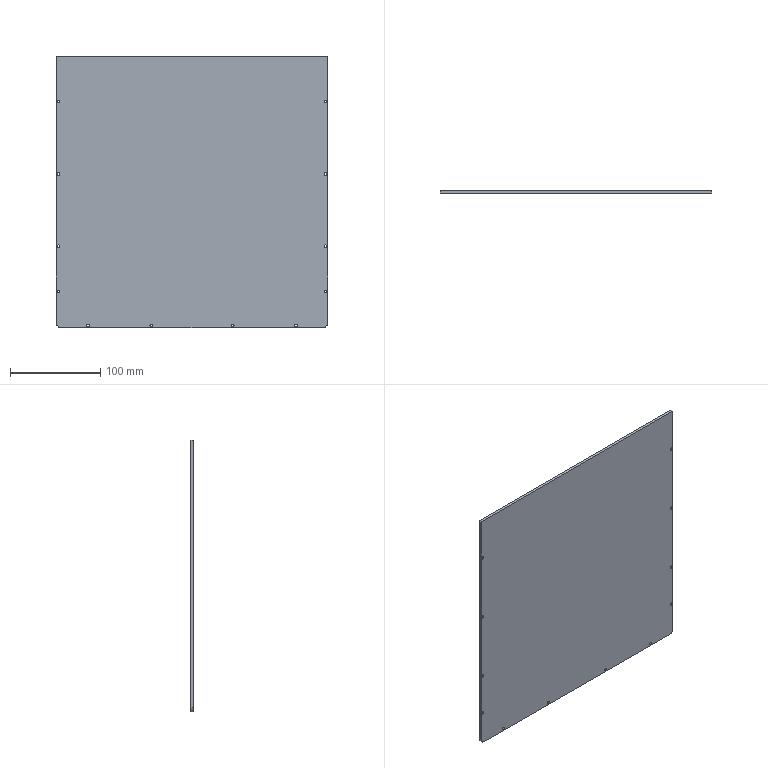Part | SolidWorks | features Extrusion 1 | 1 solid | 32 faces | box 300 x 3 x 300 mm | volume 269713 mm3 | cylinder 26 | plane 6 | commonest cylinder face diameters 3 x24 10 x2
STEP:
#1=CARTESIAN_POINT('',(147.5,3.,-61.5));
#2=VERTEX_POINT('',#1);
#3=CARTESIAN_POINT('',(147.5,3.,-58.5));
#4=VERTEX_POINT('',#3);
#5=CARTESIAN_POINT('',(147.5,3.,-60.));
#6=DIRECTION('',(0.,1.,0.));
#7=DIRECTION('',(0.,0.,-1.));
#8=AXIS2_PLACEMENT_3D('',#5,#6,#7);
#9=CIRCLE('',#8,1.5);
#10=EDGE_CURVE('',#2,#4,#9,.T.);
#11=ORIENTED_EDGE('',*,*,#10,.T.);
#12=CARTESIAN_POINT('',(147.5,0.,-58.5));
#13=VERTEX_POINT('',#12);
#14=CARTESIAN_POINT('',(147.5,3.,-58.5));
#15=DIRECTION('',(0.,-1.,0.));
#16=VECTOR('',#15,1000.);
#17=LINE('',#14,#16);
#18=EDGE_CURVE('',#4,#13,#17,.T.);
#19=ORIENTED_EDGE('',*,*,#18,.T.);
#20=CARTESIAN_POINT('',(147.5,0.,-61.5));
#21=VERTEX_POINT('',#20);
#22=CARTESIAN_POINT('',(147.5,0.,-60.));
#23=DIRECTION('',(0.,1.,0.));
#24=DIRECTION('',(0.,0.,-1.));
#25=AXIS2_PLACEMENT_3D('',#22,#23,#24);
#26=CIRCLE('',#25,1.5);
#27=EDGE_CURVE('',#21,#13,#26,.T.);
#28=ORIENTED_EDGE('',*,*,#27,.F.);
#29=CARTESIAN_POINT('',(147.5,3.,-61.5));
#30=DIRECTION('',(0.,-1.,0.));
#31=VECTOR('',#30,1000.);
#32=LINE('',#29,#31);
#33=EDGE_CURVE('',#2,#21,#32,.T.);
#34=ORIENTED_EDGE('',*,*,#33,.F.);
#35=EDGE_LOOP('',(#11,#19,#28,#34));
#36=FACE_OUTER_BOUND('',#35,.T.);
#37=CARTESIAN_POINT('',(147.5,3.,-60.));
#38=DIRECTION('',(0.,-1.,0.));
#39=DIRECTION('',(0.,0.,-1.));
#40=AXIS2_PLACEMENT_3D('',#37,#38,#39);
#41=CYLINDRICAL_SURFACE('',#40,1.5);
#42=ADVANCED_FACE('',(#36),#41,.F.);
#43=CARTESIAN_POINT('',(147.5,3.,-111.5));
#44=VERTEX_POINT('',#43);
#45=CARTESIAN_POINT('',(147.5,3.,-108.5));
#46=VERTEX_POINT('',#45);
#47=CARTESIAN_POINT('',(147.5,3.,-110.));
#48=DIRECTION('',(0.,1.,0.));
#49=DIRECTION('',(0.,0.,-1.));
#50=AXIS2_PLACEMENT_3D('',#47,#48,#49);
#51=CIRCLE('',#50,1.5);
#52=EDGE_CURVE('',#44,#46,#51,.T.);
#53=ORIENTED_EDGE('',*,*,#52,.T.);
#54=CARTESIAN_POINT('',(147.5,0.,-108.5));
#55=VERTEX_POINT('',#54);
#56=CARTESIAN_POINT('',(147.5,3.,-108.5));
#57=DIRECTION('',(0.,-1.,0.));
#58=VECTOR('',#57,1000.);
#59=LINE('',#56,#58);
#60=EDGE_CURVE('',#46,#55,#59,.T.);
#61=ORIENTED_EDGE('',*,*,#60,.T.);
#62=CARTESIAN_POINT('',(147.5,0.,-111.5));
#63=VERTEX_POINT('',#62);
#64=CARTESIAN_POINT('',(147.5,0.,-110.));
#65=DIRECTION('',(0.,1.,0.));
#66=DIRECTION('',(0.,0.,-1.));
#67=AXIS2_PLACEMENT_3D('',#64,#65,#66);
#68=CIRCLE('',#67,1.5);
#69=EDGE_CURVE('',#63,#55,#68,.T.);
#70=ORIENTED_EDGE('',*,*,#69,.F.);
#71=CARTESIAN_POINT('',(147.5,3.,-111.5));
#72=DIRECTION('',(0.,-1.,0.));
#73=VECTOR('',#72,1000.);
#74=LINE('',#71,#73);
#75=EDGE_CURVE('',#44,#63,#74,.T.);
#76=ORIENTED_EDGE('',*,*,#75,.F.);
#77=EDGE_LOOP('',(#53,#61,#70,#76));
#78=FACE_OUTER_BOUND('',#77,.T.);
#79=CARTESIAN_POINT('',(147.5,3.,-110.));
#80=DIRECTION('',(0.,-1.,0.));
#81=DIRECTION('',(0.,0.,-1.));
#82=AXIS2_PLACEMENT_3D('',#79,#80,#81);
#83=CYLINDRICAL_SURFACE('',#82,1.5);
#84=ADVANCED_FACE('',(#78),#83,.F.);
#85=CARTESIAN_POINT('',(147.5,3.,98.5));
#86=VERTEX_POINT('',#85);
#87=CARTESIAN_POINT('',(147.5,3.,101.5));
#88=VERTEX_POINT('',#87);
#89=CARTESIAN_POINT('',(147.5,3.,100.));
#90=DIRECTION('',(0.,1.,0.));
#91=DIRECTION('',(0.,0.,-1.));
#92=AXIS2_PLACEMENT_3D('',#89,#90,#91);
#93=CIRCLE('',#92,1.5);
#94=EDGE_CURVE('',#86,#88,#93,.T.);
#95=ORIENTED_EDGE('',*,*,#94,.T.);
#96=CARTESIAN_POINT('',(147.5,0.,101.5));
#97=VERTEX_POINT('',#96);
#98=CARTESIAN_POINT('',(147.5,3.,101.5));
#99=DIRECTION('',(0.,-1.,0.));
#100=VECTOR('',#99,1000.);
#101=LINE('',#98,#100);
#102=EDGE_CURVE('',#88,#97,#101,.T.);
#103=ORIENTED_EDGE('',*,*,#102,.T.);
#104=CARTESIAN_POINT('',(147.5,0.,98.5));
#105=VERTEX_POINT('',#104);
#106=CARTESIAN_POINT('',(147.5,0.,100.));
#107=DIRECTION('',(0.,1.,0.));
#108=DIRECTION('',(0.,0.,-1.));
#109=AXIS2_PLACEMENT_3D('',#106,#107,#108);
#110=CIRCLE('',#109,1.5);
#111=EDGE_CURVE('',#105,#97,#110,.T.);
#112=ORIENTED_EDGE('',*,*,#111,.F.);
#113=CARTESIAN_POINT('',(147.5,3.,98.5));
#114=DIRECTION('',(0.,-1.,0.));
#115=VECTOR('',#114,1000.);
#116=LINE('',#113,#115);
#117=EDGE_CURVE('',#86,#105,#116,.T.);
#118=ORIENTED_EDGE('',*,*,#117,.F.);
#119=EDGE_LOOP('',(#95,#103,#112,#118));
#120=FACE_OUTER_BOUND('',#119,.T.);
#121=CARTESIAN_POINT('',(147.5,3.,100.));
#122=DIRECTION('',(0.,-1.,0.));
#123=DIRECTION('',(0.,0.,-1.));
#124=AXIS2_PLACEMENT_3D('',#121,#122,#123);
#125=CYLINDRICAL_SURFACE('',#124,1.5);
#126=ADVANCED_FACE('',(#120),#125,.F.);
#127=CARTESIAN_POINT('',(147.5,3.,18.5));
#128=VERTEX_POINT('',#127);
#129=CARTESIAN_POINT('',(147.5,3.,21.5));
#130=VERTEX_POINT('',#129);
#131=CARTESIAN_POINT('',(147.5,3.,20.));
#132=DIRECTION('',(0.,1.,0.));
#133=DIRECTION('',(0.,0.,-1.));
#134=AXIS2_PLACEMENT_3D('',#131,#132,#133);
#135=CIRCLE('',#134,1.5);
#136=EDGE_CURVE('',#128,#130,#135,.T.);
#137=ORIENTED_EDGE('',*,*,#136,.T.);
#138=CARTESIAN_POINT('',(147.5,0.,21.5));
#139=VERTEX_POINT('',#138);
#140=CARTESIAN_POINT('',(147.5,3.,21.5));
#141=DIRECTION('',(0.,-1.,0.));
#142=VECTOR('',#141,1000.);
#143=LINE('',#140,#142);
#144=EDGE_CURVE('',#130,#139,#143,.T.);
#145=ORIENTED_EDGE('',*,*,#144,.T.);
#146=CARTESIAN_POINT('',(147.5,0.,18.5));
#147=VERTEX_POINT('',#146);
#148=CARTESIAN_POINT('',(147.5,0.,20.));
#149=DIRECTION('',(0.,1.,0.));
#150=DIRECTION('',(0.,0.,-1.));
#151=AXIS2_PLACEMENT_3D('',#148,#149,#150);
#152=CIRCLE('',#151,1.5);
#153=EDGE_CURVE('',#147,#139,#152,.T.);
#154=ORIENTED_EDGE('',*,*,#153,.F.);
#155=CARTESIAN_POINT('',(147.5,3.,18.5));
#156=DIRECTION('',(0.,-1.,0.));
#157=VECTOR('',#156,1000.);
#158=LINE('',#155,#157);
#159=EDGE_CURVE('',#128,#147,#158,.T.);
#160=ORIENTED_EDGE('',*,*,#159,.F.);
#161=EDGE_LOOP('',(#137,#145,#154,#160));
#162=FACE_OUTER_BOUND('',#161,.T.);
#163=CARTESIAN_POINT('',(147.5,3.,20.));
#164=DIRECTION('',(0.,-1.,0.));
#165=DIRECTION('',(0.,0.,-1.));
#166=AXIS2_PLACEMENT_3D('',#163,#164,#165);
#167=CYLINDRICAL_SURFACE('',#166,1.5);
#168=ADVANCED_FACE('',(#162),#167,.F.);
#169=CARTESIAN_POINT('',(115.,3.,-149.));
#170=VERTEX_POINT('',#169);
#171=CARTESIAN_POINT('',(115.,3.,-146.));
#172=VERTEX_POINT('',#171);
#173=CARTESIAN_POINT('',(115.,3.,-147.5));
#174=DIRECTION('',(0.,1.,0.));
#175=DIRECTION('',(0.,0.,-1.));
#176=AXIS2_PLACEMENT_3D('',#173,#174,#175);
#177=CIRCLE('',#176,1.5);
#178=EDGE_CURVE('',#170,#172,#177,.T.);
#179=ORIENTED_EDGE('',*,*,#178,.T.);
#180=CARTESIAN_POINT('',(115.,0.,-146.));
#181=VERTEX_POINT('',#180);
#182=CARTESIAN_POINT('',(115.,3.,-146.));
#183=DIRECTION('',(0.,-1.,0.));
#184=VECTOR('',#183,1000.);
#185=LINE('',#182,#184);
#186=EDGE_CURVE('',#172,#181,#185,.T.);
#187=ORIENTED_EDGE('',*,*,#186,.T.);
#188=CARTESIAN_POINT('',(115.,0.,-149.));
#189=VERTEX_POINT('',#188);
#190=CARTESIAN_POINT('',(115.,0.,-147.5));
#191=DIRECTION('',(0.,1.,0.));
#192=DIRECTION('',(0.,0.,-1.));
#193=AXIS2_PLACEMENT_3D('',#190,#191,#192);
#194=CIRCLE('',#193,1.5);
#195=EDGE_CURVE('',#189,#181,#194,.T.);
#196=ORIENTED_EDGE('',*,*,#195,.F.);
#197=CARTESIAN_POINT('',(115.,3.,-149.));
#198=DIRECTION('',(0.,-1.,0.));
#199=VECTOR('',#198,1000.);
#200=LINE('',#197,#199);
#201=EDGE_CURVE('',#170,#189,#200,.T.);
#202=ORIENTED_EDGE('',*,*,#201,.F.);
#203=EDGE_LOOP('',(#179,#187,#196,#202));
#204=FACE_OUTER_BOUND('',#203,.T.);
#205=CARTESIAN_POINT('',(115.,3.,-147.5));
#206=DIRECTION('',(0.,-1.,0.));
#207=DIRECTION('',(0.,0.,-1.));
#208=AXIS2_PLACEMENT_3D('',#205,#206,#207);
#209=CYLINDRICAL_SURFACE('',#208,1.5);
#210=ADVANCED_FACE('',(#204),#209,.F.);
#211=CARTESIAN_POINT('',(45.,3.,-149.));
#212=VERTEX_POINT('',#211);
#213=CARTESIAN_POINT('',(45.,3.,-146.));
#214=VERTEX_POINT('',#213);
#215=CARTESIAN_POINT('',(45.,3.,-147.5));
#216=DIRECTION('',(0.,1.,0.));
#217=DIRECTION('',(0.,0.,-1.));
#218=AXIS2_PLACEMENT_3D('',#215,#216,#217);
#219=CIRCLE('',#218,1.5);
#220=EDGE_CURVE('',#212,#214,#219,.T.);
#221=ORIENTED_EDGE('',*,*,#220,.T.);
#222=CARTESIAN_POINT('',(45.,0.,-146.));
#223=VERTEX_POINT('',#222);
#224=CARTESIAN_POINT('',(45.,3.,-146.));
#225=DIRECTION('',(0.,-1.,0.));
#226=VECTOR('',#225,1000.);
#227=LINE('',#224,#226);
#228=EDGE_CURVE('',#214,#223,#227,.T.);
#229=ORIENTED_EDGE('',*,*,#228,.T.);
#230=CARTESIAN_POINT('',(45.,0.,-149.));
#231=VERTEX_POINT('',#230);
#232=CARTESIAN_POINT('',(45.,0.,-147.5));
#233=DIRECTION('',(0.,1.,0.));
#234=DIRECTION('',(0.,0.,-1.));
#235=AXIS2_PLACEMENT_3D('',#232,#233,#234);
#236=CIRCLE('',#235,1.5);
#237=EDGE_CURVE('',#231,#223,#236,.T.);
#238=ORIENTED_EDGE('',*,*,#237,.F.);
#239=CARTESIAN_POINT('',(45.,3.,-149.));
#240=DIRECTION('',(0.,-1.,0.));
#241=VECTOR('',#240,1000.);
#242=LINE('',#239,#241);
#243=EDGE_CURVE('',#212,#231,#242,.T.);
#244=ORIENTED_EDGE('',*,*,#243,.F.);
#245=EDGE_LOOP('',(#221,#229,#238,#244));
#246=FACE_OUTER_BOUND('',#245,.T.);
#247=CARTESIAN_POINT('',(45.,3.,-147.5));
#248=DIRECTION('',(0.,-1.,0.));
#249=DIRECTION('',(0.,0.,-1.));
#250=AXIS2_PLACEMENT_3D('',#247,#248,#249);
#251=CYLINDRICAL_SURFACE('',#250,1.5);
#252=ADVANCED_FACE('',(#246),#251,.F.);
#253=CARTESIAN_POINT('',(-45.,3.,-149.));
#254=VERTEX_POINT('',#253);
#255=CARTESIAN_POINT('',(-45.,3.,-146.));
#256=VERTEX_POINT('',#255);
#257=CARTESIAN_POINT('',(-45.,3.,-147.5));
#258=DIRECTION('',(0.,1.,0.));
#259=DIRECTION('',(0.,0.,1.));
#260=AXIS2_PLACEMENT_3D('',#257,#258,#259);
#261=CIRCLE('',#260,1.5);
#262=EDGE_CURVE('',#254,#256,#261,.T.);
#263=ORIENTED_EDGE('',*,*,#262,.T.);
#264=CARTESIAN_POINT('',(-45.,0.,-146.));
#265=VERTEX_POINT('',#264);
#266=CARTESIAN_POINT('',(-45.,3.,-146.));
#267=DIRECTION('',(0.,-1.,0.));
#268=VECTOR('',#267,1000.);
#269=LINE('',#266,#268);
#270=EDGE_CURVE('',#256,#265,#269,.T.);
#271=ORIENTED_EDGE('',*,*,#270,.T.);
#272=CARTESIAN_POINT('',(-45.,0.,-149.));
#273=VERTEX_POINT('',#272);
#274=CARTESIAN_POINT('',(-45.,0.,-147.5));
#275=DIRECTION('',(0.,1.,0.));
#276=DIRECTION('',(0.,0.,1.));
#277=AXIS2_PLACEMENT_3D('',#274,#275,#276);
#278=CIRCLE('',#277,1.5);
#279=EDGE_CURVE('',#273,#265,#278,.T.);
#280=ORIENTED_EDGE('',*,*,#279,.F.);
#281=CARTESIAN_POINT('',(-45.,3.,-149.));
#282=DIRECTION('',(0.,-1.,0.));
#283=VECTOR('',#282,1000.);
#284=LINE('',#281,#283);
#285=EDGE_CURVE('',#254,#273,#284,.T.);
#286=ORIENTED_EDGE('',*,*,#285,.F.);
#287=EDGE_LOOP('',(#263,#271,#280,#286));
#288=FACE_OUTER_BOUND('',#287,.T.);
#289=CARTESIAN_POINT('',(-45.,3.,-147.5));
#290=DIRECTION('',(0.,-1.,0.));
#291=DIRECTION('',(0.,0.,-1.));
#292=AXIS2_PLACEMENT_3D('',#289,#290,#291);
#293=CYLINDRICAL_SURFACE('',#292,1.5);
#294=ADVANCED_FACE('',(#288),#293,.F.);
#295=CARTESIAN_POINT('',(-115.,3.,-149.));
#296=VERTEX_POINT('',#295);
#297=CARTESIAN_POINT('',(-115.,3.,-146.));
#298=VERTEX_POINT('',#297);
#299=CARTESIAN_POINT('',(-115.,3.,-147.5));
#300=DIRECTION('',(0.,1.,0.));
#301=DIRECTION('',(0.,0.,1.));
#302=AXIS2_PLACEMENT_3D('',#299,#300,#301);
#303=CIRCLE('',#302,1.5);
#304=EDGE_CURVE('',#296,#298,#303,.T.);
#305=ORIENTED_EDGE('',*,*,#304,.T.);
#306=CARTESIAN_POINT('',(-115.,0.,-146.));
#307=VERTEX_POINT('',#306);
#308=CARTESIAN_POINT('',(-115.,3.,-146.));
#309=DIRECTION('',(0.,-1.,0.));
#310=VECTOR('',#309,1000.);
#311=LINE('',#308,#310);
#312=EDGE_CURVE('',#298,#307,#311,.T.);
#313=ORIENTED_EDGE('',*,*,#312,.T.);
#314=CARTESIAN_POINT('',(-115.,0.,-149.));
#315=VERTEX_POINT('',#314);
#316=CARTESIAN_POINT('',(-115.,0.,-147.5));
#317=DIRECTION('',(0.,1.,0.));
#318=DIRECTION('',(0.,0.,1.));
#319=AXIS2_PLACEMENT_3D('',#316,#317,#318);
#320=CIRCLE('',#319,1.5);
#321=EDGE_CURVE('',#315,#307,#320,.T.);
#322=ORIENTED_EDGE('',*,*,#321,.F.);
#323=CARTESIAN_POINT('',(-115.,3.,-149.));
#324=DIRECTION('',(0.,-1.,0.));
#325=VECTOR('',#324,1000.);
#326=LINE('',#323,#325);
#327=EDGE_CURVE('',#296,#315,#326,.T.);
#328=ORIENTED_EDGE('',*,*,#327,.F.);
#329=EDGE_LOOP('',(#305,#313,#322,#328));
#330=FACE_OUTER_BOUND('',#329,.T.);
#331=CARTESIAN_POINT('',(-115.,3.,-147.5));
#332=DIRECTION('',(0.,-1.,0.));
#333=DIRECTION('',(0.,0.,-1.));
#334=AXIS2_PLACEMENT_3D('',#331,#332,#333);
#335=CYLINDRICAL_SURFACE('',#334,1.5);
#336=ADVANCED_FACE('',(#330),#335,.F.);
#337=CARTESIAN_POINT('',(-147.5,3.,-111.5));
#338=VERTEX_POINT('',#337);
#339=CARTESIAN_POINT('',(-147.5,3.,-108.5));
#340=VERTEX_POINT('',#339);
#341=CARTESIAN_POINT('',(-147.5,3.,-110.));
#342=DIRECTION('',(0.,1.,0.));
#343=DIRECTION('',(0.,0.,1.));
#344=AXIS2_PLACEMENT_3D('',#341,#342,#343);
#345=CIRCLE('',#344,1.5);
#346=EDGE_CURVE('',#338,#340,#345,.T.);
#347=ORIENTED_EDGE('',*,*,#346,.T.);
#348=CARTESIAN_POINT('',(-147.5,0.,-108.5));
#349=VERTEX_POINT('',#348);
#350=CARTESIAN_POINT('',(-147.5,3.,-108.5));
#351=DIRECTION('',(0.,-1.,0.));
#352=VECTOR('',#351,1000.);
#353=LINE('',#350,#352);
#354=EDGE_CURVE('',#340,#349,#353,.T.);
#355=ORIENTED_EDGE('',*,*,#354,.T.);
#356=CARTESIAN_POINT('',(-147.5,0.,-111.5));
#357=VERTEX_POINT('',#356);
#358=CARTESIAN_POINT('',(-147.5,0.,-110.));
#359=DIRECTION('',(0.,1.,0.));
#360=DIRECTION('',(0.,0.,1.));
#361=AXIS2_PLACEMENT_3D('',#358,#359,#360);
#362=CIRCLE('',#361,1.5);
#363=EDGE_CURVE('',#357,#349,#362,.T.);
#364=ORIENTED_EDGE('',*,*,#363,.F.);
#365=CARTESIAN_POINT('',(-147.5,3.,-111.5));
#366=DIRECTION('',(0.,-1.,0.));
#367=VECTOR('',#366,1000.);
#368=LINE('',#365,#367);
#369=EDGE_CURVE('',#338,#357,#368,.T.);
#370=ORIENTED_EDGE('',*,*,#369,.F.);
#371=EDGE_LOOP('',(#347,#355,#364,#370));
#372=FACE_OUTER_BOUND('',#371,.T.);
#373=CARTESIAN_POINT('',(-147.5,3.,-110.));
#374=DIRECTION('',(0.,-1.,0.));
#375=DIRECTION('',(0.,0.,-1.));
#376=AXIS2_PLACEMENT_3D('',#373,#374,#375);
#377=CYLINDRICAL_SURFACE('',#376,1.5);
#378=ADVANCED_FACE('',(#372),#377,.F.);
#379=CARTESIAN_POINT('',(-147.5,3.,-61.5));
#380=VERTEX_POINT('',#379);
#381=CARTESIAN_POINT('',(-147.5,3.,-58.5));
#382=VERTEX_POINT('',#381);
#383=CARTESIAN_POINT('',(-147.5,3.,-60.));
#384=DIRECTION('',(0.,1.,0.));
#385=DIRECTION('',(0.,0.,1.));
#386=AXIS2_PLACEMENT_3D('',#383,#384,#385);
#387=CIRCLE('',#386,1.5);
#388=EDGE_CURVE('',#380,#382,#387,.T.);
#389=ORIENTED_EDGE('',*,*,#388,.T.);
#390=CARTESIAN_POINT('',(-147.5,0.,-58.5));
#391=VERTEX_POINT('',#390);
#392=CARTESIAN_POINT('',(-147.5,3.,-58.5));
#393=DIRECTION('',(0.,-1.,0.));
#394=VECTOR('',#393,1000.);
#395=LINE('',#392,#394);
#396=EDGE_CURVE('',#382,#391,#395,.T.);
#397=ORIENTED_EDGE('',*,*,#396,.T.);
#398=CARTESIAN_POINT('',(-147.5,0.,-61.5));
#399=VERTEX_POINT('',#398);
#400=CARTESIAN_POINT('',(-147.5,0.,-60.));
#401=DIRECTION('',(0.,1.,0.));
#402=DIRECTION('',(0.,0.,1.));
#403=AXIS2_PLACEMENT_3D('',#400,#401,#402);
#404=CIRCLE('',#403,1.5);
#405=EDGE_CURVE('',#399,#391,#404,.T.);
#406=ORIENTED_EDGE('',*,*,#405,.F.);
#407=CARTESIAN_POINT('',(-147.5,3.,-61.5));
#408=DIRECTION('',(0.,-1.,0.));
#409=VECTOR('',#408,1000.);
#410=LINE('',#407,#409);
#411=EDGE_CURVE('',#380,#399,#410,.T.);
#412=ORIENTED_EDGE('',*,*,#411,.F.);
#413=EDGE_LOOP('',(#389,#397,#406,#412));
#414=FACE_OUTER_BOUND('',#413,.T.);
#415=CARTESIAN_POINT('',(-147.5,3.,-60.));
#416=DIRECTION('',(0.,-1.,0.));
#417=DIRECTION('',(0.,0.,-1.));
#418=AXIS2_PLACEMENT_3D('',#415,#416,#417);
#419=CYLINDRICAL_SURFACE('',#418,1.5);
#420=ADVANCED_FACE('',(#414),#419,.F.);
#421=CARTESIAN_POINT('',(-147.5,3.,18.5));
#422=VERTEX_POINT('',#421);
#423=CARTESIAN_POINT('',(-147.5,3.,21.5));
#424=VERTEX_POINT('',#423);
#425=CARTESIAN_POINT('',(-147.5,3.,20.));
#426=DIRECTION('',(0.,1.,0.));
#427=DIRECTION('',(0.,0.,1.));
#428=AXIS2_PLACEMENT_3D('',#425,#426,#427);
#429=CIRCLE('',#428,1.5);
#430=EDGE_CURVE('',#422,#424,#429,.T.);
#431=ORIENTED_EDGE('',*,*,#430,.T.);
#432=CARTESIAN_POINT('',(-147.5,0.,21.5));
#433=VERTEX_POINT('',#432);
#434=CARTESIAN_POINT('',(-147.5,3.,21.5));
#435=DIRECTION('',(0.,-1.,0.));
#436=VECTOR('',#435,1000.);
#437=LINE('',#434,#436);
#438=EDGE_CURVE('',#424,#433,#437,.T.);
#439=ORIENTED_EDGE('',*,*,#438,.T.);
#440=CARTESIAN_POINT('',(-147.5,0.,18.5));
#441=VERTEX_POINT('',#440);
#442=CARTESIAN_POINT('',(-147.5,0.,20.));
#443=DIRECTION('',(0.,1.,0.));
#444=DIRECTION('',(0.,0.,1.));
#445=AXIS2_PLACEMENT_3D('',#442,#443,#444);
#446=CIRCLE('',#445,1.5);
#447=EDGE_CURVE('',#441,#433,#446,.T.);
#448=ORIENTED_EDGE('',*,*,#447,.F.);
#449=CARTESIAN_POINT('',(-147.5,3.,18.5));
#450=DIRECTION('',(0.,-1.,0.));
#451=VECTOR('',#450,1000.);
#452=LINE('',#449,#451);
#453=EDGE_CURVE('',#422,#441,#452,.T.);
#454=ORIENTED_EDGE('',*,*,#453,.F.);
#455=EDGE_LOOP('',(#431,#439,#448,#454));
#456=FACE_OUTER_BOUND('',#455,.T.);
#457=CARTESIAN_POINT('',(-147.5,3.,20.));
#458=DIRECTION('',(0.,-1.,0.));
#459=DIRECTION('',(0.,0.,-1.));
#460=AXIS2_PLACEMENT_3D('',#457,#458,#459);
#461=CYLINDRICAL_SURFACE('',#460,1.5);
#462=ADVANCED_FACE('',(#456),#461,.F.);
#463=CARTESIAN_POINT('',(-147.5,3.,98.5));
#464=VERTEX_POINT('',#463);
#465=CARTESIAN_POINT('',(-147.5,3.,101.5));
#466=VERTEX_POINT('',#465);
#467=CARTESIAN_POINT('',(-147.5,3.,100.));
#468=DIRECTION('',(0.,1.,0.));
#469=DIRECTION('',(0.,0.,1.));
#470=AXIS2_PLACEMENT_3D('',#467,#468,#469);
#471=CIRCLE('',#470,1.5);
#472=EDGE_CURVE('',#464,#466,#471,.T.);
#473=ORIENTED_EDGE('',*,*,#472,.T.);
#474=CARTESIAN_POINT('',(-147.5,0.,101.5));
#475=VERTEX_POINT('',#474);
#476=CARTESIAN_POINT('',(-147.5,3.,101.5));
#477=DIRECTION('',(0.,-1.,0.));
#478=VECTOR('',#477,1000.);
#479=LINE('',#476,#478);
#480=EDGE_CURVE('',#466,#475,#479,.T.);
#481=ORIENTED_EDGE('',*,*,#480,.T.);
#482=CARTESIAN_POINT('',(-147.5,0.,98.5));
#483=VERTEX_POINT('',#482);
#484=CARTESIAN_POINT('',(-147.5,0.,100.));
#485=DIRECTION('',(0.,1.,0.));
#486=DIRECTION('',(0.,0.,1.));
#487=AXIS2_PLACEMENT_3D('',#484,#485,#486);
#488=CIRCLE('',#487,1.5);
#489=EDGE_CURVE('',#483,#475,#488,.T.);
#490=ORIENTED_EDGE('',*,*,#489,.F.);
#491=CARTESIAN_POINT('',(-147.5,3.,98.5));
#492=DIRECTION('',(0.,-1.,0.));
#493=VECTOR('',#492,1000.);
#494=LINE('',#491,#493);
#495=EDGE_CURVE('',#464,#483,#494,.T.);
#496=ORIENTED_EDGE('',*,*,#495,.F.);
#497=EDGE_LOOP('',(#473,#481,#490,#496));
#498=FACE_OUTER_BOUND('',#497,.T.);
#499=CARTESIAN_POINT('',(-147.5,3.,100.));
#500=DIRECTION('',(0.,-1.,0.));
#501=DIRECTION('',(0.,0.,-1.));
#502=AXIS2_PLACEMENT_3D('',#499,#500,#501);
#503=CYLINDRICAL_SURFACE('',#502,1.5);
#504=ADVANCED_FACE('',(#498),#503,.F.);
#505=CARTESIAN_POINT('',(-150.,3.,-145.));
#506=VERTEX_POINT('',#505);
#507=CARTESIAN_POINT('',(-150.,3.,150.));
#508=VERTEX_POINT('',#507);
#509=CARTESIAN_POINT('',(-150.,3.,150.));
#510=DIRECTION('',(0.,0.,1.));
#511=VECTOR('',#510,1000.);
#512=LINE('',#509,#511);
#513=EDGE_CURVE('',#506,#508,#512,.T.);
#514=ORIENTED_EDGE('',*,*,#513,.T.);
#515=CARTESIAN_POINT('',(150.,3.,150.));
#516=VERTEX_POINT('',#515);
#517=CARTESIAN_POINT('',(-150.,3.,150.));
#518=DIRECTION('',(1.,0.,0.));
#519=VECTOR('',#518,1000.);
#520=LINE('',#517,#519);
#521=EDGE_CURVE('',#508,#516,#520,.T.);
#522=ORIENTED_EDGE('',*,*,#521,.T.);
#523=CARTESIAN_POINT('',(150.,3.,-145.));
#524=VERTEX_POINT('',#523);
#525=CARTESIAN_POINT('',(150.,3.,150.));
#526=DIRECTION('',(0.,0.,-1.));
#527=VECTOR('',#526,1000.);
#528=LINE('',#525,#527);
#529=EDGE_CURVE('',#516,#524,#528,.T.);
#530=ORIENTED_EDGE('',*,*,#529,.T.);
#531=CARTESIAN_POINT('',(145.,3.,-150.));
#532=VERTEX_POINT('',#531);
#533=CARTESIAN_POINT('',(145.,3.,-145.));
#534=DIRECTION('',(0.,1.,0.));
#535=DIRECTION('',(0.,0.,-1.));
#536=AXIS2_PLACEMENT_3D('',#533,#534,#535);
#537=CIRCLE('',#536,5.);
#538=EDGE_CURVE('',#524,#532,#537,.T.);
#539=ORIENTED_EDGE('',*,*,#538,.T.);
#540=CARTESIAN_POINT('',(-145.,3.,-150.));
#541=VERTEX_POINT('',#540);
#542=CARTESIAN_POINT('',(-145.,3.,-150.));
#543=DIRECTION('',(-1.,0.,0.));
#544=VECTOR('',#543,1000.);
#545=LINE('',#542,#544);
#546=EDGE_CURVE('',#532,#541,#545,.T.);
#547=ORIENTED_EDGE('',*,*,#546,.T.);
#548=CARTESIAN_POINT('',(-145.,3.,-145.));
#549=DIRECTION('',(0.,1.,0.));
#550=DIRECTION('',(0.,0.,-1.));
#551=AXIS2_PLACEMENT_3D('',#548,#549,#550);
#552=CIRCLE('',#551,5.);
#553=EDGE_CURVE('',#541,#506,#552,.T.);
#554=ORIENTED_EDGE('',*,*,#553,.T.);
#555=EDGE_LOOP('',(#514,#522,#530,#539,#547,#554));
#556=FACE_OUTER_BOUND('',#555,.T.);
#557=ORIENTED_EDGE('',*,*,#472,.F.);
#558=CARTESIAN_POINT('',(-147.5,3.,100.));
#559=DIRECTION('',(0.,1.,0.));
#560=DIRECTION('',(0.,0.,1.));
#561=AXIS2_PLACEMENT_3D('',#558,#559,#560);
#562=CIRCLE('',#561,1.5);
#563=EDGE_CURVE('',#466,#464,#562,.T.);
#564=ORIENTED_EDGE('',*,*,#563,.F.);
#565=EDGE_LOOP('',(#557,#564));
#566=FACE_BOUND('',#565,.T.);
#567=ORIENTED_EDGE('',*,*,#430,.F.);
#568=CARTESIAN_POINT('',(-147.5,3.,20.));
#569=DIRECTION('',(0.,1.,0.));
#570=DIRECTION('',(0.,0.,1.));
#571=AXIS2_PLACEMENT_3D('',#568,#569,#570);
#572=CIRCLE('',#571,1.5);
#573=EDGE_CURVE('',#424,#422,#572,.T.);
#574=ORIENTED_EDGE('',*,*,#573,.F.);
#575=EDGE_LOOP('',(#567,#574));
#576=FACE_BOUND('',#575,.T.);
#577=ORIENTED_EDGE('',*,*,#388,.F.);
#578=CARTESIAN_POINT('',(-147.5,3.,-60.));
#579=DIRECTION('',(0.,1.,0.));
#580=DIRECTION('',(0.,0.,1.));
#581=AXIS2_PLACEMENT_3D('',#578,#579,#580);
#582=CIRCLE('',#581,1.5);
#583=EDGE_CURVE('',#382,#380,#582,.T.);
#584=ORIENTED_EDGE('',*,*,#583,.F.);
#585=EDGE_LOOP('',(#577,#584));
#586=FACE_BOUND('',#585,.T.);
#587=ORIENTED_EDGE('',*,*,#346,.F.);
#588=CARTESIAN_POINT('',(-147.5,3.,-110.));
#589=DIRECTION('',(0.,1.,0.));
#590=DIRECTION('',(0.,0.,1.));
#591=AXIS2_PLACEMENT_3D('',#588,#589,#590);
#592=CIRCLE('',#591,1.5);
#593=EDGE_CURVE('',#340,#338,#592,.T.);
#594=ORIENTED_EDGE('',*,*,#593,.F.);
#595=EDGE_LOOP('',(#587,#594));
#596=FACE_BOUND('',#595,.T.);
#597=ORIENTED_EDGE('',*,*,#304,.F.);
#598=CARTESIAN_POINT('',(-115.,3.,-147.5));
#599=DIRECTION('',(0.,1.,0.));
#600=DIRECTION('',(0.,0.,1.));
#601=AXIS2_PLACEMENT_3D('',#598,#599,#600);
#602=CIRCLE('',#601,1.5);
#603=EDGE_CURVE('',#298,#296,#602,.T.);
#604=ORIENTED_EDGE('',*,*,#603,.F.);
#605=EDGE_LOOP('',(#597,#604));
#606=FACE_BOUND('',#605,.T.);
#607=ORIENTED_EDGE('',*,*,#262,.F.);
#608=CARTESIAN_POINT('',(-45.,3.,-147.5));
#609=DIRECTION('',(0.,1.,0.));
#610=DIRECTION('',(0.,0.,1.));
#611=AXIS2_PLACEMENT_3D('',#608,#609,#610);
#612=CIRCLE('',#611,1.5);
#613=EDGE_CURVE('',#256,#254,#612,.T.);
#614=ORIENTED_EDGE('',*,*,#613,.F.);
#615=EDGE_LOOP('',(#607,#614));
#616=FACE_BOUND('',#615,.T.);
#617=ORIENTED_EDGE('',*,*,#220,.F.);
#618=CARTESIAN_POINT('',(45.,3.,-147.5));
#619=DIRECTION('',(0.,1.,0.));
#620=DIRECTION('',(0.,0.,-1.));
#621=AXIS2_PLACEMENT_3D('',#618,#619,#620);
#622=CIRCLE('',#621,1.5);
#623=EDGE_CURVE('',#214,#212,#622,.T.);
#624=ORIENTED_EDGE('',*,*,#623,.F.);
#625=EDGE_LOOP('',(#617,#624));
#626=FACE_BOUND('',#625,.T.);
#627=ORIENTED_EDGE('',*,*,#178,.F.);
#628=CARTESIAN_POINT('',(115.,3.,-147.5));
#629=DIRECTION('',(0.,1.,0.));
#630=DIRECTION('',(0.,0.,-1.));
#631=AXIS2_PLACEMENT_3D('',#628,#629,#630);
#632=CIRCLE('',#631,1.5);
#633=EDGE_CURVE('',#172,#170,#632,.T.);
#634=ORIENTED_EDGE('',*,*,#633,.F.);
#635=EDGE_LOOP('',(#627,#634));
#636=FACE_BOUND('',#635,.T.);
#637=ORIENTED_EDGE('',*,*,#136,.F.);
#638=CARTESIAN_POINT('',(147.5,3.,20.));
#639=DIRECTION('',(0.,1.,0.));
#640=DIRECTION('',(0.,0.,-1.));
#641=AXIS2_PLACEMENT_3D('',#638,#639,#640);
#642=CIRCLE('',#641,1.5);
#643=EDGE_CURVE('',#130,#128,#642,.T.);
#644=ORIENTED_EDGE('',*,*,#643,.F.);
#645=EDGE_LOOP('',(#637,#644));
#646=FACE_BOUND('',#645,.T.);
#647=ORIENTED_EDGE('',*,*,#94,.F.);
#648=CARTESIAN_POINT('',(147.5,3.,100.));
#649=DIRECTION('',(0.,1.,0.));
#650=DIRECTION('',(0.,0.,-1.));
#651=AXIS2_PLACEMENT_3D('',#648,#649,#650);
#652=CIRCLE('',#651,1.5);
#653=EDGE_CURVE('',#88,#86,#652,.T.);
#654=ORIENTED_EDGE('',*,*,#653,.F.);
#655=EDGE_LOOP('',(#647,#654));
#656=FACE_BOUND('',#655,.T.);
#657=ORIENTED_EDGE('',*,*,#52,.F.);
#658=CARTESIAN_POINT('',(147.5,3.,-110.));
#659=DIRECTION('',(0.,1.,0.));
#660=DIRECTION('',(0.,0.,-1.));
#661=AXIS2_PLACEMENT_3D('',#658,#659,#660);
#662=CIRCLE('',#661,1.5);
#663=EDGE_CURVE('',#46,#44,#662,.T.);
#664=ORIENTED_EDGE('',*,*,#663,.F.);
#665=EDGE_LOOP('',(#657,#664));
#666=FACE_BOUND('',#665,.T.);
#667=ORIENTED_EDGE('',*,*,#10,.F.);
#668=CARTESIAN_POINT('',(147.5,3.,-60.));
#669=DIRECTION('',(0.,1.,0.));
#670=DIRECTION('',(0.,0.,-1.));
#671=AXIS2_PLACEMENT_3D('',#668,#669,#670);
#672=CIRCLE('',#671,1.5);
#673=EDGE_CURVE('',#4,#2,#672,.T.);
#674=ORIENTED_EDGE('',*,*,#673,.F.);
#675=EDGE_LOOP('',(#667,#674));
#676=FACE_BOUND('',#675,.T.);
#677=CARTESIAN_POINT('',(-145.,3.,-145.));
#678=DIRECTION('',(0.,-1.,0.));
#679=DIRECTION('',(0.,0.,-1.));
#680=AXIS2_PLACEMENT_3D('',#677,#678,#679);
#681=PLANE('',#680);
#682=ADVANCED_FACE('',(#556,#566,#576,#586,#596,#606,#616,#626,#636,#646,#656,#666,#676),#681,.F.);
#683=ORIENTED_EDGE('',*,*,#69,.T.);
#684=CARTESIAN_POINT('',(147.5,0.,-110.));
#685=DIRECTION('',(0.,1.,0.));
#686=DIRECTION('',(0.,0.,-1.));
#687=AXIS2_PLACEMENT_3D('',#684,#685,#686);
#688=CIRCLE('',#687,1.5);
#689=EDGE_CURVE('',#55,#63,#688,.T.);
#690=ORIENTED_EDGE('',*,*,#689,.T.);
#691=EDGE_LOOP('',(#683,#690));
#692=FACE_BOUND('',#691,.T.);
#693=ORIENTED_EDGE('',*,*,#153,.T.);
#694=CARTESIAN_POINT('',(147.5,0.,20.));
#695=DIRECTION('',(0.,1.,0.));
#696=DIRECTION('',(0.,0.,-1.));
#697=AXIS2_PLACEMENT_3D('',#694,#695,#696);
#698=CIRCLE('',#697,1.5);
#699=EDGE_CURVE('',#139,#147,#698,.T.);
#700=ORIENTED_EDGE('',*,*,#699,.T.);
#701=EDGE_LOOP('',(#693,#700));
#702=FACE_BOUND('',#701,.T.);
#703=ORIENTED_EDGE('',*,*,#237,.T.);
#704=CARTESIAN_POINT('',(45.,0.,-147.5));
#705=DIRECTION('',(0.,1.,0.));
#706=DIRECTION('',(0.,0.,-1.));
#707=AXIS2_PLACEMENT_3D('',#704,#705,#706);
#708=CIRCLE('',#707,1.5);
#709=EDGE_CURVE('',#223,#231,#708,.T.);
#710=ORIENTED_EDGE('',*,*,#709,.T.);
#711=EDGE_LOOP('',(#703,#710));
#712=FACE_BOUND('',#711,.T.);
#713=ORIENTED_EDGE('',*,*,#321,.T.);
#714=CARTESIAN_POINT('',(-115.,0.,-147.5));
#715=DIRECTION('',(0.,1.,0.));
#716=DIRECTION('',(0.,0.,1.));
#717=AXIS2_PLACEMENT_3D('',#714,#715,#716);
#718=CIRCLE('',#717,1.5);
#719=EDGE_CURVE('',#307,#315,#718,.T.);
#720=ORIENTED_EDGE('',*,*,#719,.T.);
#721=EDGE_LOOP('',(#713,#720));
#722=FACE_BOUND('',#721,.T.);
#723=ORIENTED_EDGE('',*,*,#405,.T.);
#724=CARTESIAN_POINT('',(-147.5,0.,-60.));
#725=DIRECTION('',(0.,1.,0.));
#726=DIRECTION('',(0.,0.,1.));
#727=AXIS2_PLACEMENT_3D('',#724,#725,#726);
#728=CIRCLE('',#727,1.5);
#729=EDGE_CURVE('',#391,#399,#728,.T.);
#730=ORIENTED_EDGE('',*,*,#729,.T.);
#731=EDGE_LOOP('',(#723,#730));
#732=FACE_BOUND('',#731,.T.);
#733=ORIENTED_EDGE('',*,*,#489,.T.);
#734=CARTESIAN_POINT('',(-147.5,0.,100.));
#735=DIRECTION('',(0.,1.,0.));
#736=DIRECTION('',(0.,0.,1.));
#737=AXIS2_PLACEMENT_3D('',#734,#735,#736);
#738=CIRCLE('',#737,1.5);
#739=EDGE_CURVE('',#475,#483,#738,.T.);
#740=ORIENTED_EDGE('',*,*,#739,.T.);
#741=EDGE_LOOP('',(#733,#740));
#742=FACE_BOUND('',#741,.T.);
#743=CARTESIAN_POINT('',(-150.,0.,-145.));
#744=VERTEX_POINT('',#743);
#745=CARTESIAN_POINT('',(-150.,0.,150.));
#746=VERTEX_POINT('',#745);
#747=CARTESIAN_POINT('',(-150.,0.,150.));
#748=DIRECTION('',(0.,0.,1.));
#749=VECTOR('',#748,1000.);
#750=LINE('',#747,#749);
#751=EDGE_CURVE('',#744,#746,#750,.T.);
#752=ORIENTED_EDGE('',*,*,#751,.F.);
#753=CARTESIAN_POINT('',(-145.,0.,-150.));
#754=VERTEX_POINT('',#753);
#755=CARTESIAN_POINT('',(-145.,0.,-145.));
#756=DIRECTION('',(0.,1.,0.));
#757=DIRECTION('',(0.,0.,-1.));
#758=AXIS2_PLACEMENT_3D('',#755,#756,#757);
#759=CIRCLE('',#758,5.);
#760=EDGE_CURVE('',#754,#744,#759,.T.);
#761=ORIENTED_EDGE('',*,*,#760,.F.);
#762=CARTESIAN_POINT('',(145.,0.,-150.));
#763=VERTEX_POINT('',#762);
#764=CARTESIAN_POINT('',(-145.,0.,-150.));
#765=DIRECTION('',(-1.,0.,0.));
#766=VECTOR('',#765,1000.);
#767=LINE('',#764,#766);
#768=EDGE_CURVE('',#763,#754,#767,.T.);
#769=ORIENTED_EDGE('',*,*,#768,.F.);
#770=CARTESIAN_POINT('',(150.,0.,-145.));
#771=VERTEX_POINT('',#770);
#772=CARTESIAN_POINT('',(145.,0.,-145.));
#773=DIRECTION('',(0.,1.,0.));
#774=DIRECTION('',(0.,0.,-1.));
#775=AXIS2_PLACEMENT_3D('',#772,#773,#774);
#776=CIRCLE('',#775,5.);
#777=EDGE_CURVE('',#771,#763,#776,.T.);
#778=ORIENTED_EDGE('',*,*,#777,.F.);
#779=CARTESIAN_POINT('',(150.,0.,150.));
#780=VERTEX_POINT('',#779);
#781=CARTESIAN_POINT('',(150.,0.,150.));
#782=DIRECTION('',(0.,0.,-1.));
#783=VECTOR('',#782,1000.);
#784=LINE('',#781,#783);
#785=EDGE_CURVE('',#780,#771,#784,.T.);
#786=ORIENTED_EDGE('',*,*,#785,.F.);
#787=CARTESIAN_POINT('',(-150.,0.,150.));
#788=DIRECTION('',(1.,0.,0.));
#789=VECTOR('',#788,1000.);
#790=LINE('',#787,#789);
#791=EDGE_CURVE('',#746,#780,#790,.T.);
#792=ORIENTED_EDGE('',*,*,#791,.F.);
#793=EDGE_LOOP('',(#752,#761,#769,#778,#786,#792));
#794=FACE_OUTER_BOUND('',#793,.T.);
#795=ORIENTED_EDGE('',*,*,#447,.T.);
#796=CARTESIAN_POINT('',(-147.5,0.,20.));
#797=DIRECTION('',(0.,1.,0.));
#798=DIRECTION('',(0.,0.,1.));
#799=AXIS2_PLACEMENT_3D('',#796,#797,#798);
#800=CIRCLE('',#799,1.5);
#801=EDGE_CURVE('',#433,#441,#800,.T.);
#802=ORIENTED_EDGE('',*,*,#801,.T.);
#803=EDGE_LOOP('',(#795,#802));
#804=FACE_BOUND('',#803,.T.);
#805=ORIENTED_EDGE('',*,*,#363,.T.);
#806=CARTESIAN_POINT('',(-147.5,0.,-110.));
#807=DIRECTION('',(0.,1.,0.));
#808=DIRECTION('',(0.,0.,1.));
#809=AXIS2_PLACEMENT_3D('',#806,#807,#808);
#810=CIRCLE('',#809,1.5);
#811=EDGE_CURVE('',#349,#357,#810,.T.);
#812=ORIENTED_EDGE('',*,*,#811,.T.);
#813=EDGE_LOOP('',(#805,#812));
#814=FACE_BOUND('',#813,.T.);
#815=ORIENTED_EDGE('',*,*,#279,.T.);
#816=CARTESIAN_POINT('',(-45.,0.,-147.5));
#817=DIRECTION('',(0.,1.,0.));
#818=DIRECTION('',(0.,0.,1.));
#819=AXIS2_PLACEMENT_3D('',#816,#817,#818);
#820=CIRCLE('',#819,1.5);
#821=EDGE_CURVE('',#265,#273,#820,.T.);
#822=ORIENTED_EDGE('',*,*,#821,.T.);
#823=EDGE_LOOP('',(#815,#822));
#824=FACE_BOUND('',#823,.T.);
#825=ORIENTED_EDGE('',*,*,#195,.T.);
#826=CARTESIAN_POINT('',(115.,0.,-147.5));
#827=DIRECTION('',(0.,1.,0.));
#828=DIRECTION('',(0.,0.,-1.));
#829=AXIS2_PLACEMENT_3D('',#826,#827,#828);
#830=CIRCLE('',#829,1.5);
#831=EDGE_CURVE('',#181,#189,#830,.T.);
#832=ORIENTED_EDGE('',*,*,#831,.T.);
#833=EDGE_LOOP('',(#825,#832));
#834=FACE_BOUND('',#833,.T.);
#835=ORIENTED_EDGE('',*,*,#111,.T.);
#836=CARTESIAN_POINT('',(147.5,0.,100.));
#837=DIRECTION('',(0.,1.,0.));
#838=DIRECTION('',(0.,0.,-1.));
#839=AXIS2_PLACEMENT_3D('',#836,#837,#838);
#840=CIRCLE('',#839,1.5);
#841=EDGE_CURVE('',#97,#105,#840,.T.);
#842=ORIENTED_EDGE('',*,*,#841,.T.);
#843=EDGE_LOOP('',(#835,#842));
#844=FACE_BOUND('',#843,.T.);
#845=ORIENTED_EDGE('',*,*,#27,.T.);
#846=CARTESIAN_POINT('',(147.5,0.,-60.));
#847=DIRECTION('',(0.,1.,0.));
#848=DIRECTION('',(0.,0.,-1.));
#849=AXIS2_PLACEMENT_3D('',#846,#847,#848);
#850=CIRCLE('',#849,1.5);
#851=EDGE_CURVE('',#13,#21,#850,.T.);
#852=ORIENTED_EDGE('',*,*,#851,.T.);
#853=EDGE_LOOP('',(#845,#852));
#854=FACE_BOUND('',#853,.T.);
#855=CARTESIAN_POINT('',(-145.,0.,-145.));
#856=DIRECTION('',(0.,-1.,0.));
#857=DIRECTION('',(0.,0.,-1.));
#858=AXIS2_PLACEMENT_3D('',#855,#856,#857);
#859=PLANE('',#858);
#860=ADVANCED_FACE('',(#692,#702,#712,#722,#732,#742,#794,#804,#814,#824,#834,#844,#854),#859,.T.);
#861=ORIENTED_EDGE('',*,*,#751,.T.);
#862=CARTESIAN_POINT('',(-150.,3.,150.));
#863=DIRECTION('',(0.,-1.,0.));
#864=VECTOR('',#863,1000.);
#865=LINE('',#862,#864);
#866=EDGE_CURVE('',#508,#746,#865,.T.);
#867=ORIENTED_EDGE('',*,*,#866,.F.);
#868=ORIENTED_EDGE('',*,*,#513,.F.);
#869=CARTESIAN_POINT('',(-150.,3.,-145.));
#870=DIRECTION('',(0.,-1.,0.));
#871=VECTOR('',#870,1000.);
#872=LINE('',#869,#871);
#873=EDGE_CURVE('',#506,#744,#872,.T.);
#874=ORIENTED_EDGE('',*,*,#873,.T.);
#875=EDGE_LOOP('',(#861,#867,#868,#874));
#876=FACE_OUTER_BOUND('',#875,.T.);
#877=CARTESIAN_POINT('',(-150.,3.,150.));
#878=DIRECTION('',(1.,0.,0.));
#879=DIRECTION('',(0.,0.,-1.));
#880=AXIS2_PLACEMENT_3D('',#877,#878,#879);
#881=PLANE('',#880);
#882=ADVANCED_FACE('',(#876),#881,.F.);
#883=ORIENTED_EDGE('',*,*,#791,.T.);
#884=CARTESIAN_POINT('',(150.,3.,150.));
#885=DIRECTION('',(0.,-1.,0.));
#886=VECTOR('',#885,1000.);
#887=LINE('',#884,#886);
#888=EDGE_CURVE('',#516,#780,#887,.T.);
#889=ORIENTED_EDGE('',*,*,#888,.F.);
#890=ORIENTED_EDGE('',*,*,#521,.F.);
#891=ORIENTED_EDGE('',*,*,#866,.T.);
#892=EDGE_LOOP('',(#883,#889,#890,#891));
#893=FACE_OUTER_BOUND('',#892,.T.);
#894=CARTESIAN_POINT('',(-150.,3.,150.));
#895=DIRECTION('',(0.,0.,-1.));
#896=DIRECTION('',(-1.,0.,0.));
#897=AXIS2_PLACEMENT_3D('',#894,#895,#896);
#898=PLANE('',#897);
#899=ADVANCED_FACE('',(#893),#898,.F.);
#900=ORIENTED_EDGE('',*,*,#785,.T.);
#901=CARTESIAN_POINT('',(150.,3.,-145.));
#902=DIRECTION('',(0.,-1.,0.));
#903=VECTOR('',#902,1000.);
#904=LINE('',#901,#903);
#905=EDGE_CURVE('',#524,#771,#904,.T.);
#906=ORIENTED_EDGE('',*,*,#905,.F.);
#907=ORIENTED_EDGE('',*,*,#529,.F.);
#908=ORIENTED_EDGE('',*,*,#888,.T.);
#909=EDGE_LOOP('',(#900,#906,#907,#908));
#910=FACE_OUTER_BOUND('',#909,.T.);
#911=CARTESIAN_POINT('',(150.,3.,150.));
#912=DIRECTION('',(-1.,0.,0.));
#913=DIRECTION('',(0.,0.,1.));
#914=AXIS2_PLACEMENT_3D('',#911,#912,#913);
#915=PLANE('',#914);
#916=ADVANCED_FACE('',(#910),#915,.F.);
#917=ORIENTED_EDGE('',*,*,#777,.T.);
#918=CARTESIAN_POINT('',(145.,3.,-150.));
#919=DIRECTION('',(0.,-1.,0.));
#920=VECTOR('',#919,1000.);
#921=LINE('',#918,#920);
#922=EDGE_CURVE('',#532,#763,#921,.T.);
#923=ORIENTED_EDGE('',*,*,#922,.F.);
#924=ORIENTED_EDGE('',*,*,#538,.F.);
#925=ORIENTED_EDGE('',*,*,#905,.T.);
#926=EDGE_LOOP('',(#917,#923,#924,#925));
#927=FACE_OUTER_BOUND('',#926,.T.);
#928=CARTESIAN_POINT('',(145.,3.,-145.));
#929=DIRECTION('',(0.,-1.,0.));
#930=DIRECTION('',(0.,0.,-1.));
#931=AXIS2_PLACEMENT_3D('',#928,#929,#930);
#932=CYLINDRICAL_SURFACE('',#931,5.);
#933=ADVANCED_FACE('',(#927),#932,.T.);
#934=ORIENTED_EDGE('',*,*,#768,.T.);
#935=CARTESIAN_POINT('',(-145.,3.,-150.));
#936=DIRECTION('',(0.,-1.,0.));
#937=VECTOR('',#936,1000.);
#938=LINE('',#935,#937);
#939=EDGE_CURVE('',#541,#754,#938,.T.);
#940=ORIENTED_EDGE('',*,*,#939,.F.);
#941=ORIENTED_EDGE('',*,*,#546,.F.);
#942=ORIENTED_EDGE('',*,*,#922,.T.);
#943=EDGE_LOOP('',(#934,#940,#941,#942));
#944=FACE_OUTER_BOUND('',#943,.T.);
#945=CARTESIAN_POINT('',(-145.,3.,-150.));
#946=DIRECTION('',(0.,0.,1.));
#947=DIRECTION('',(1.,0.,0.));
#948=AXIS2_PLACEMENT_3D('',#945,#946,#947);
#949=PLANE('',#948);
#950=ADVANCED_FACE('',(#944),#949,.F.);
#951=ORIENTED_EDGE('',*,*,#760,.T.);
#952=ORIENTED_EDGE('',*,*,#873,.F.);
#953=ORIENTED_EDGE('',*,*,#553,.F.);
#954=ORIENTED_EDGE('',*,*,#939,.T.);
#955=EDGE_LOOP('',(#951,#952,#953,#954));
#956=FACE_OUTER_BOUND('',#955,.T.);
#957=CARTESIAN_POINT('',(-145.,3.,-145.));
#958=DIRECTION('',(0.,-1.,0.));
#959=DIRECTION('',(0.,0.,-1.));
#960=AXIS2_PLACEMENT_3D('',#957,#958,#959);
#961=CYLINDRICAL_SURFACE('',#960,5.);
#962=ADVANCED_FACE('',(#956),#961,.T.);
#963=ORIENTED_EDGE('',*,*,#480,.F.);
#964=ORIENTED_EDGE('',*,*,#563,.T.);
#965=ORIENTED_EDGE('',*,*,#495,.T.);
#966=ORIENTED_EDGE('',*,*,#739,.F.);
#967=EDGE_LOOP('',(#963,#964,#965,#966));
#968=FACE_OUTER_BOUND('',#967,.T.);
#969=CARTESIAN_POINT('',(-147.5,3.,100.));
#970=DIRECTION('',(0.,-1.,0.));
#971=DIRECTION('',(0.,0.,-1.));
#972=AXIS2_PLACEMENT_3D('',#969,#970,#971);
#973=CYLINDRICAL_SURFACE('',#972,1.5);
#974=ADVANCED_FACE('',(#968),#973,.F.);
#975=ORIENTED_EDGE('',*,*,#438,.F.);
#976=ORIENTED_EDGE('',*,*,#573,.T.);
#977=ORIENTED_EDGE('',*,*,#453,.T.);
#978=ORIENTED_EDGE('',*,*,#801,.F.);
#979=EDGE_LOOP('',(#975,#976,#977,#978));
#980=FACE_OUTER_BOUND('',#979,.T.);
#981=CARTESIAN_POINT('',(-147.5,3.,20.));
#982=DIRECTION('',(0.,-1.,0.));
#983=DIRECTION('',(0.,0.,-1.));
#984=AXIS2_PLACEMENT_3D('',#981,#982,#983);
#985=CYLINDRICAL_SURFACE('',#984,1.5);
#986=ADVANCED_FACE('',(#980),#985,.F.);
#987=ORIENTED_EDGE('',*,*,#396,.F.);
#988=ORIENTED_EDGE('',*,*,#583,.T.);
#989=ORIENTED_EDGE('',*,*,#411,.T.);
#990=ORIENTED_EDGE('',*,*,#729,.F.);
#991=EDGE_LOOP('',(#987,#988,#989,#990));
#992=FACE_OUTER_BOUND('',#991,.T.);
#993=CARTESIAN_POINT('',(-147.5,3.,-60.));
#994=DIRECTION('',(0.,-1.,0.));
#995=DIRECTION('',(0.,0.,-1.));
#996=AXIS2_PLACEMENT_3D('',#993,#994,#995);
#997=CYLINDRICAL_SURFACE('',#996,1.5);
#998=ADVANCED_FACE('',(#992),#997,.F.);
#999=ORIENTED_EDGE('',*,*,#354,.F.);
#1000=ORIENTED_EDGE('',*,*,#593,.T.);
#1001=ORIENTED_EDGE('',*,*,#369,.T.);
#1002=ORIENTED_EDGE('',*,*,#811,.F.);
#1003=EDGE_LOOP('',(#999,#1000,#1001,#1002));
#1004=FACE_OUTER_BOUND('',#1003,.T.);
#1005=CARTESIAN_POINT('',(-147.5,3.,-110.));
#1006=DIRECTION('',(0.,-1.,0.));
#1007=DIRECTION('',(0.,0.,-1.));
#1008=AXIS2_PLACEMENT_3D('',#1005,#1006,#1007);
#1009=CYLINDRICAL_SURFACE('',#1008,1.5);
#1010=ADVANCED_FACE('',(#1004),#1009,.F.);
#1011=ORIENTED_EDGE('',*,*,#312,.F.);
#1012=ORIENTED_EDGE('',*,*,#603,.T.);
#1013=ORIENTED_EDGE('',*,*,#327,.T.);
#1014=ORIENTED_EDGE('',*,*,#719,.F.);
#1015=EDGE_LOOP('',(#1011,#1012,#1013,#1014));
#1016=FACE_OUTER_BOUND('',#1015,.T.);
#1017=CARTESIAN_POINT('',(-115.,3.,-147.5));
#1018=DIRECTION('',(0.,-1.,0.));
#1019=DIRECTION('',(0.,0.,-1.));
#1020=AXIS2_PLACEMENT_3D('',#1017,#1018,#1019);
#1021=CYLINDRICAL_SURFACE('',#1020,1.5);
#1022=ADVANCED_FACE('',(#1016),#1021,.F.);
#1023=ORIENTED_EDGE('',*,*,#270,.F.);
#1024=ORIENTED_EDGE('',*,*,#613,.T.);
#1025=ORIENTED_EDGE('',*,*,#285,.T.);
#1026=ORIENTED_EDGE('',*,*,#821,.F.);
#1027=EDGE_LOOP('',(#1023,#1024,#1025,#1026));
#1028=FACE_OUTER_BOUND('',#1027,.T.);
#1029=CARTESIAN_POINT('',(-45.,3.,-147.5));
#1030=DIRECTION('',(0.,-1.,0.));
#1031=DIRECTION('',(0.,0.,-1.));
#1032=AXIS2_PLACEMENT_3D('',#1029,#1030,#1031);
#1033=CYLINDRICAL_SURFACE('',#1032,1.5);
#1034=ADVANCED_FACE('',(#1028),#1033,.F.);
#1035=ORIENTED_EDGE('',*,*,#228,.F.);
#1036=ORIENTED_EDGE('',*,*,#623,.T.);
#1037=ORIENTED_EDGE('',*,*,#243,.T.);
#1038=ORIENTED_EDGE('',*,*,#709,.F.);
#1039=EDGE_LOOP('',(#1035,#1036,#1037,#1038));
#1040=FACE_OUTER_BOUND('',#1039,.T.);
#1041=CARTESIAN_POINT('',(45.,3.,-147.5));
#1042=DIRECTION('',(0.,-1.,0.));
#1043=DIRECTION('',(0.,0.,-1.));
#1044=AXIS2_PLACEMENT_3D('',#1041,#1042,#1043);
#1045=CYLINDRICAL_SURFACE('',#1044,1.5);
#1046=ADVANCED_FACE('',(#1040),#1045,.F.);
#1047=ORIENTED_EDGE('',*,*,#186,.F.);
#1048=ORIENTED_EDGE('',*,*,#633,.T.);
#1049=ORIENTED_EDGE('',*,*,#201,.T.);
#1050=ORIENTED_EDGE('',*,*,#831,.F.);
#1051=EDGE_LOOP('',(#1047,#1048,#1049,#1050));
#1052=FACE_OUTER_BOUND('',#1051,.T.);
#1053=CARTESIAN_POINT('',(115.,3.,-147.5));
#1054=DIRECTION('',(0.,-1.,0.));
#1055=DIRECTION('',(0.,0.,-1.));
#1056=AXIS2_PLACEMENT_3D('',#1053,#1054,#1055);
#1057=CYLINDRICAL_SURFACE('',#1056,1.5);
#1058=ADVANCED_FACE('',(#1052),#1057,.F.);
#1059=ORIENTED_EDGE('',*,*,#144,.F.);
#1060=ORIENTED_EDGE('',*,*,#643,.T.);
#1061=ORIENTED_EDGE('',*,*,#159,.T.);
#1062=ORIENTED_EDGE('',*,*,#699,.F.);
#1063=EDGE_LOOP('',(#1059,#1060,#1061,#1062));
#1064=FACE_OUTER_BOUND('',#1063,.T.);
#1065=CARTESIAN_POINT('',(147.5,3.,20.));
#1066=DIRECTION('',(0.,-1.,0.));
#1067=DIRECTION('',(0.,0.,-1.));
#1068=AXIS2_PLACEMENT_3D('',#1065,#1066,#1067);
#1069=CYLINDRICAL_SURFACE('',#1068,1.5);
#1070=ADVANCED_FACE('',(#1064),#1069,.F.);
#1071=ORIENTED_EDGE('',*,*,#102,.F.);
#1072=ORIENTED_EDGE('',*,*,#653,.T.);
#1073=ORIENTED_EDGE('',*,*,#117,.T.);
#1074=ORIENTED_EDGE('',*,*,#841,.F.);
#1075=EDGE_LOOP('',(#1071,#1072,#1073,#1074));
#1076=FACE_OUTER_BOUND('',#1075,.T.);
#1077=CARTESIAN_POINT('',(147.5,3.,100.));
#1078=DIRECTION('',(0.,-1.,0.));
#1079=DIRECTION('',(0.,0.,-1.));
#1080=AXIS2_PLACEMENT_3D('',#1077,#1078,#1079);
#1081=CYLINDRICAL_SURFACE('',#1080,1.5);
#1082=ADVANCED_FACE('',(#1076),#1081,.F.);
#1083=ORIENTED_EDGE('',*,*,#60,.F.);
#1084=ORIENTED_EDGE('',*,*,#663,.T.);
#1085=ORIENTED_EDGE('',*,*,#75,.T.);
#1086=ORIENTED_EDGE('',*,*,#689,.F.);
#1087=EDGE_LOOP('',(#1083,#1084,#1085,#1086));
#1088=FACE_OUTER_BOUND('',#1087,.T.);
#1089=CARTESIAN_POINT('',(147.5,3.,-110.));
#1090=DIRECTION('',(0.,-1.,0.));
#1091=DIRECTION('',(0.,0.,-1.));
#1092=AXIS2_PLACEMENT_3D('',#1089,#1090,#1091);
#1093=CYLINDRICAL_SURFACE('',#1092,1.5);
#1094=ADVANCED_FACE('',(#1088),#1093,.F.);
#1095=ORIENTED_EDGE('',*,*,#18,.F.);
#1096=ORIENTED_EDGE('',*,*,#673,.T.);
#1097=ORIENTED_EDGE('',*,*,#33,.T.);
#1098=ORIENTED_EDGE('',*,*,#851,.F.);
#1099=EDGE_LOOP('',(#1095,#1096,#1097,#1098));
#1100=FACE_OUTER_BOUND('',#1099,.T.);
#1101=CARTESIAN_POINT('',(147.5,3.,-60.));
#1102=DIRECTION('',(0.,-1.,0.));
#1103=DIRECTION('',(0.,0.,-1.));
#1104=AXIS2_PLACEMENT_3D('',#1101,#1102,#1103);
#1105=CYLINDRICAL_SURFACE('',#1104,1.5);
#1106=ADVANCED_FACE('',(#1100),#1105,.F.);
#1107=CLOSED_SHELL('',(#42,#84,#126,#168,#210,#252,#294,#336,#378,#420,#462,#504,#682,#860,#882,#899,#916,#933,#950,#962,#974,#986,#998,#1010,#1022,#1034,#1046,#1058,#1070,#1082,#1094,#1106));
#1108=MANIFOLD_SOLID_BREP('',#1107);
#1109=CARTESIAN_POINT('',(0.,0.,0.));
#1110=DIRECTION('',(0.,0.,1.));
#1111=DIRECTION('',(1.,0.,0.));
#1112=AXIS2_PLACEMENT_3D('',#1109,#1110,#1111);
#1113=(LENGTH_UNIT()NAMED_UNIT(*)SI_UNIT(.MILLI.,.METRE.));
#1114=UNCERTAINTY_MEASURE_WITH_UNIT(LENGTH_MEASURE(0.00001),#1113,'','');
#1115=(NAMED_UNIT(*)PLANE_ANGLE_UNIT()SI_UNIT($,.RADIAN.));
#1116=(NAMED_UNIT(*)SI_UNIT($,.STERADIAN.)SOLID_ANGLE_UNIT());
#1117=(GEOMETRIC_REPRESENTATION_CONTEXT(3)GLOBAL_UNCERTAINTY_ASSIGNED_CONTEXT((#1114))GLOBAL_UNIT_ASSIGNED_CONTEXT((#1113,#1115,#1116))REPRESENTATION_CONTEXT('',''));
#1118=ADVANCED_BREP_SHAPE_REPRESENTATION('',(#1108,#1112),#1117);